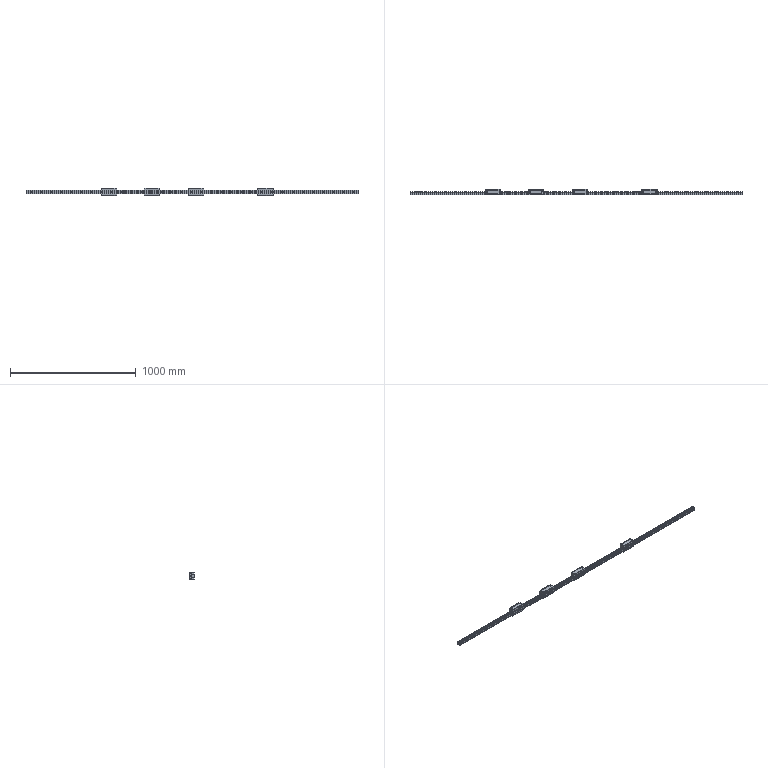Part | SolidWorks | 21 solids | 3028 faces | volume 2381123 mm3 | plane 1817 | cylinder 962 | cone 192 | spline 57 | commonest cylinder face diameters 1.2 x260 0.194 x136 1.6 x86 5.66 x84 0.097 x72 9 x66